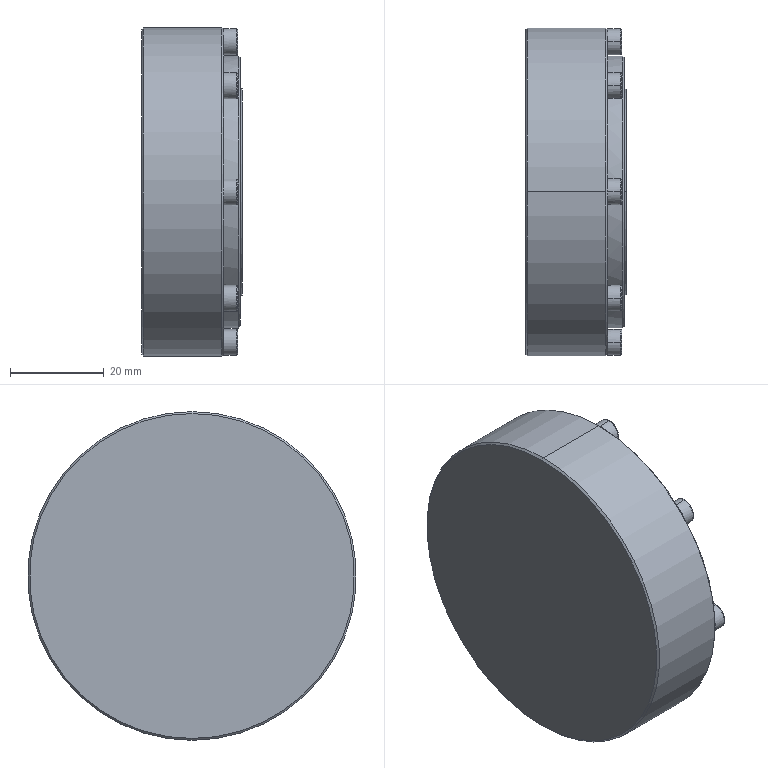Part | STEP file | ASND-0110-IRB120_3-58_IRC5_Link5_rev0-1 | 1 solid | 267 faces | box 21.5 x 70 x 70 mm | volume 66105 mm3 | cylinder 132 | plane 86 | cone 31 | torus 18 | commonest cylinder face diameters 0.2 x96 5.5 x16 44 x4 40 x2 45.4 x2 46.22 x2